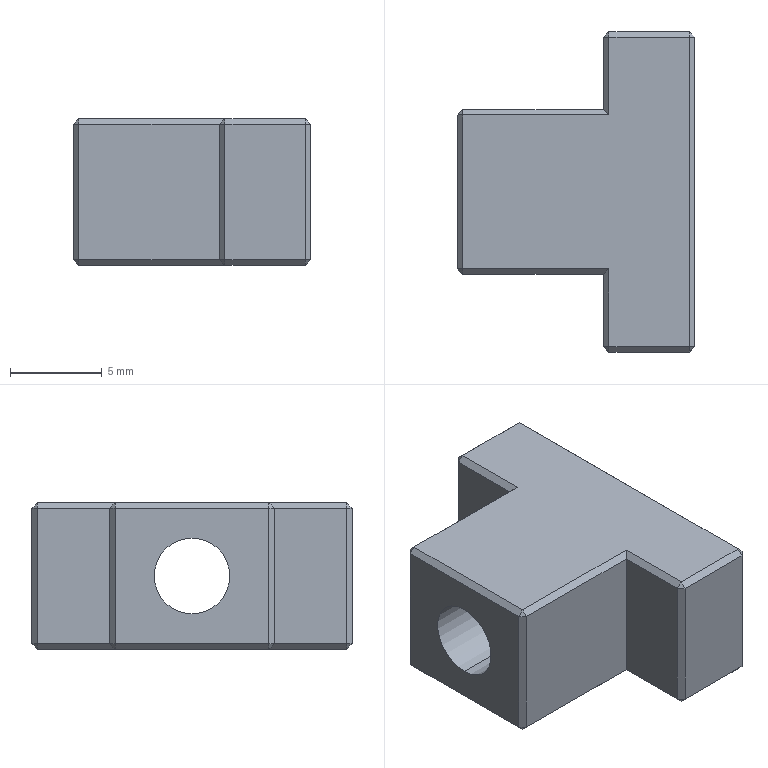Part | STEP file | A036 | 1 solid | 46 faces | box 13 x 17.5 x 8 mm | volume 1094 mm3 | plane 44 | cylinder 2 | commonest cylinder face diameters 4.134 x2